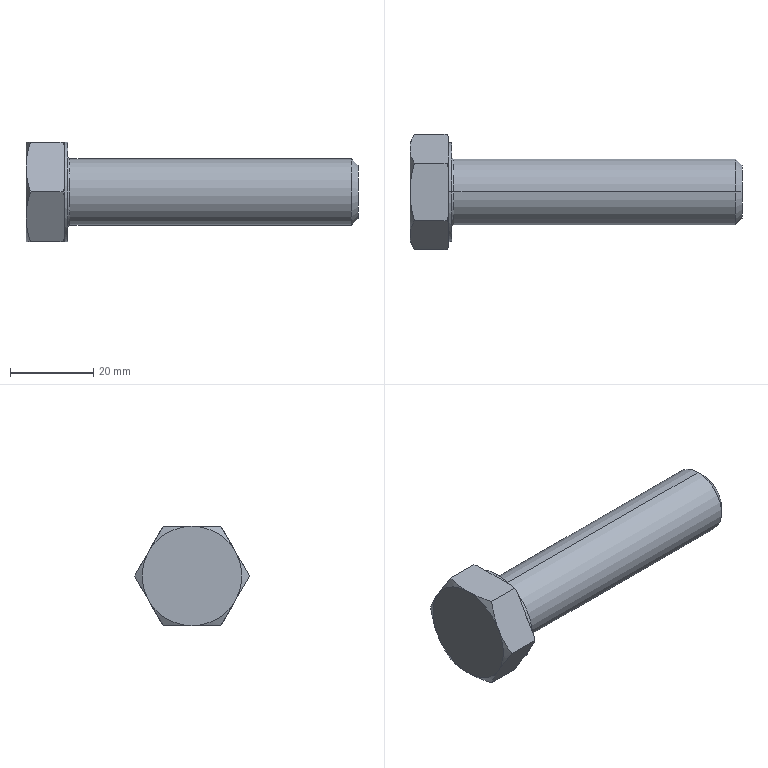Part | STEP file | 1 solid | 35 faces | box 80 x 27.713 x 24 mm | volume 18955 mm3 | plane 15 | cone 14 | cylinder 4 | spline 2 | commonest cylinder face diameters 16 x2 24 x2